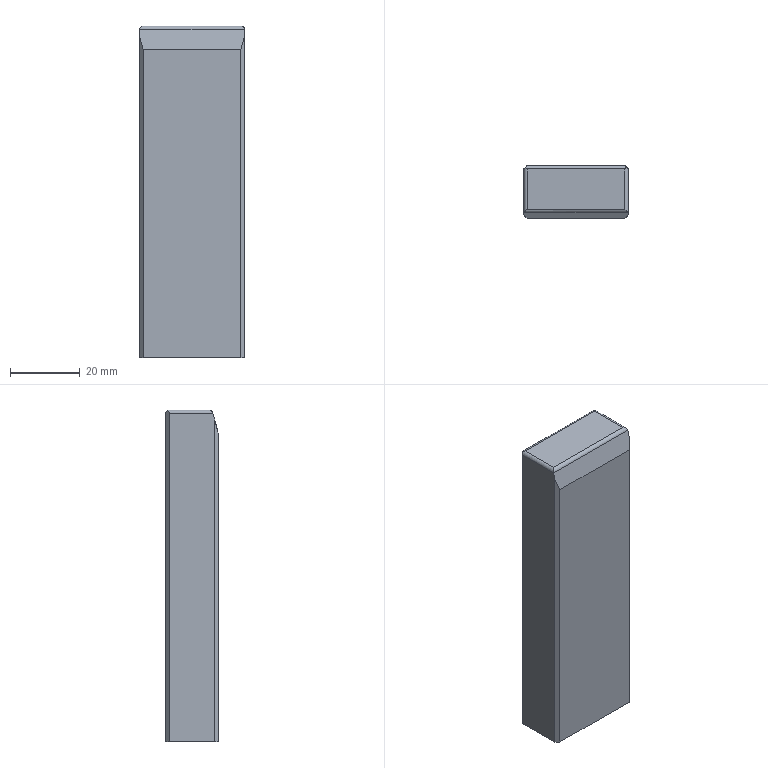Part | STEP file | chot cam | 1 solid | 19 faces | box 30 x 15 x 95 mm | volume 41659 mm3 | plane 11 | cylinder 6 | cone 2 | commonest cylinder face diameters 2 x4 6.647 x2